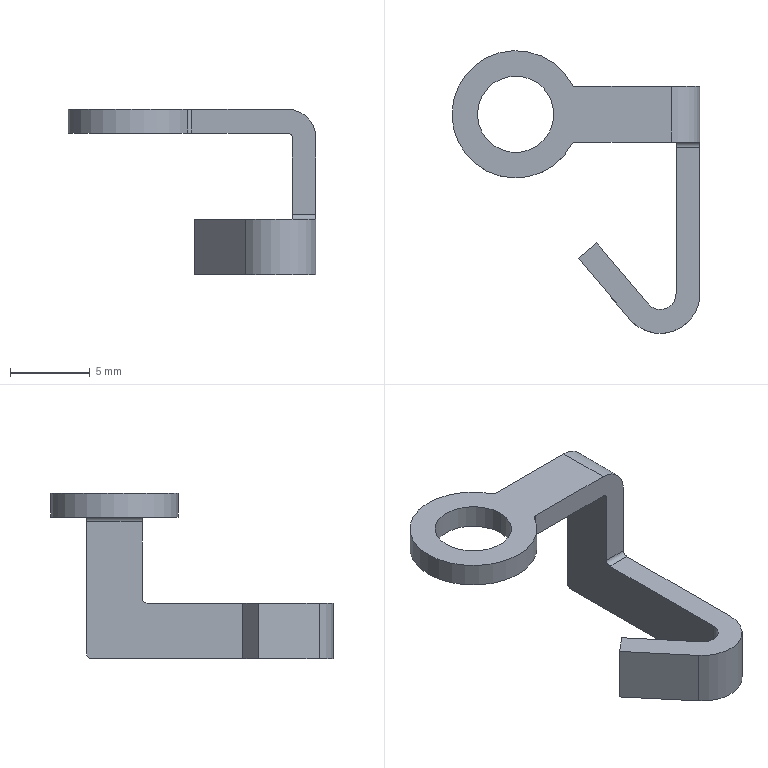Part | STEP file | TQ-DD-1105-THTerminalE1010_デフォルト | 1 solid | 22 faces | box 15.586 x 17.763 x 10.4 mm | volume 231.793 mm3 | cylinder 11 | plane 11 | commonest cylinder face diameters 0.6 x5 4.8 x2 2 x1 3.6 x1 5 x1 8 x1
STEP:
#1=CARTESIAN_POINT('',(2.4,0.,0.));
#2=VERTEX_POINT('',#1);
#3=CARTESIAN_POINT('',(-2.4,0.,0.));
#4=VERTEX_POINT('',#3);
#5=CARTESIAN_POINT('',(0.,0.,0.));
#6=DIRECTION('',(0.,0.,-1.));
#7=DIRECTION('',(1.,0.,0.));
#8=AXIS2_PLACEMENT_3D('',#5,#6,#7);
#9=CIRCLE('',#8,2.4);
#10=EDGE_CURVE('',#2,#4,#9,.T.);
#11=ORIENTED_EDGE('',*,*,#10,.T.);
#12=CARTESIAN_POINT('',(-2.4,0.,1.5));
#13=VERTEX_POINT('',#12);
#14=CARTESIAN_POINT('',(-2.4,0.,0.75));
#15=DIRECTION('',(0.,0.,1.));
#16=VECTOR('',#15,1000.);
#17=LINE('',#14,#16);
#18=EDGE_CURVE('',#4,#13,#17,.T.);
#19=ORIENTED_EDGE('',*,*,#18,.T.);
#20=CARTESIAN_POINT('',(2.4,0.,1.5));
#21=VERTEX_POINT('',#20);
#22=CARTESIAN_POINT('',(0.,0.,1.5));
#23=DIRECTION('',(0.,0.,-1.));
#24=DIRECTION('',(1.,0.,0.));
#25=AXIS2_PLACEMENT_3D('',#22,#23,#24);
#26=CIRCLE('',#25,2.4);
#27=EDGE_CURVE('',#21,#13,#26,.T.);
#28=ORIENTED_EDGE('',*,*,#27,.F.);
#29=CARTESIAN_POINT('',(2.4,0.,0.75));
#30=DIRECTION('',(0.,0.,1.));
#31=VECTOR('',#30,1000.);
#32=LINE('',#29,#31);
#33=EDGE_CURVE('',#2,#21,#32,.T.);
#34=ORIENTED_EDGE('',*,*,#33,.F.);
#35=EDGE_LOOP('',(#11,#19,#28,#34));
#36=FACE_OUTER_BOUND('',#35,.T.);
#37=CARTESIAN_POINT('',(0.,0.,0.75));
#38=DIRECTION('',(0.,0.,1.));
#39=DIRECTION('',(1.,0.,0.));
#40=AXIS2_PLACEMENT_3D('',#37,#38,#39);
#41=CYLINDRICAL_SURFACE('',#40,2.4);
#42=ADVANCED_FACE('',(#36),#41,.F.);
#43=CARTESIAN_POINT('',(10.086,-11.263,-8.9));
#44=VERTEX_POINT('',#43);
#45=CARTESIAN_POINT('',(10.086,1.45,-8.9));
#46=VERTEX_POINT('',#45);
#47=CARTESIAN_POINT('',(10.086,1.75,-8.9));
#48=DIRECTION('',(0.,1.,0.));
#49=VECTOR('',#48,1000.);
#50=LINE('',#47,#49);
#51=EDGE_CURVE('',#44,#46,#50,.T.);
#52=ORIENTED_EDGE('',*,*,#51,.F.);
#53=CARTESIAN_POINT('',(10.086,-11.263,-5.4));
#54=VERTEX_POINT('',#53);
#55=CARTESIAN_POINT('',(10.086,-11.263,-8.9));
#56=DIRECTION('',(0.,0.,-1.));
#57=VECTOR('',#56,1000.);
#58=LINE('',#55,#57);
#59=EDGE_CURVE('',#54,#44,#58,.T.);
#60=ORIENTED_EDGE('',*,*,#59,.F.);
#61=CARTESIAN_POINT('',(10.086,-2.05,-5.4));
#62=VERTEX_POINT('',#61);
#63=CARTESIAN_POINT('',(10.086,1.75,-5.4));
#64=DIRECTION('',(0.,-1.,0.));
#65=VECTOR('',#64,1000.);
#66=LINE('',#63,#65);
#67=EDGE_CURVE('',#62,#54,#66,.T.);
#68=ORIENTED_EDGE('',*,*,#67,.F.);
#69=CARTESIAN_POINT('',(10.086,-1.75,-5.1));
#70=VERTEX_POINT('',#69);
#71=CARTESIAN_POINT('',(10.086,-2.05,-5.1));
#72=DIRECTION('',(1.,0.,0.));
#73=DIRECTION('',(0.,0.,1.));
#74=AXIS2_PLACEMENT_3D('',#71,#72,#73);
#75=CIRCLE('',#74,0.3);
#76=EDGE_CURVE('',#62,#70,#75,.T.);
#77=ORIENTED_EDGE('',*,*,#76,.T.);
#78=CARTESIAN_POINT('',(10.086,-1.75,-0.3));
#79=VERTEX_POINT('',#78);
#80=CARTESIAN_POINT('',(10.086,-1.75,-8.9));
#81=DIRECTION('',(0.,0.,-1.));
#82=VECTOR('',#81,1000.);
#83=LINE('',#80,#82);
#84=EDGE_CURVE('',#79,#70,#83,.T.);
#85=ORIENTED_EDGE('',*,*,#84,.F.);
#86=CARTESIAN_POINT('',(10.086,1.75,-0.3));
#87=VERTEX_POINT('',#86);
#88=CARTESIAN_POINT('',(10.086,1.75,-0.3));
#89=DIRECTION('',(0.,-1.,0.));
#90=VECTOR('',#89,1000.);
#91=LINE('',#88,#90);
#92=EDGE_CURVE('',#87,#79,#91,.T.);
#93=ORIENTED_EDGE('',*,*,#92,.F.);
#94=CARTESIAN_POINT('',(10.086,1.75,-8.6));
#95=VERTEX_POINT('',#94);
#96=CARTESIAN_POINT('',(10.086,1.75,-8.9));
#97=DIRECTION('',(0.,0.,1.));
#98=VECTOR('',#97,1000.);
#99=LINE('',#96,#98);
#100=EDGE_CURVE('',#95,#87,#99,.T.);
#101=ORIENTED_EDGE('',*,*,#100,.F.);
#102=CARTESIAN_POINT('',(10.086,1.45,-8.6));
#103=DIRECTION('',(1.,0.,0.));
#104=DIRECTION('',(0.,0.,-1.));
#105=AXIS2_PLACEMENT_3D('',#102,#103,#104);
#106=CIRCLE('',#105,0.3);
#107=EDGE_CURVE('',#46,#95,#106,.T.);
#108=ORIENTED_EDGE('',*,*,#107,.F.);
#109=EDGE_LOOP('',(#52,#60,#68,#77,#85,#93,#101,#108));
#110=FACE_OUTER_BOUND('',#109,.T.);
#111=CARTESIAN_POINT('',(10.086,1.75,-8.9));
#112=DIRECTION('',(1.,0.,0.));
#113=DIRECTION('',(0.,0.,-1.));
#114=AXIS2_PLACEMENT_3D('',#111,#112,#113);
#115=PLANE('',#114);
#116=ADVANCED_FACE('',(#110),#115,.F.);
#117=ORIENTED_EDGE('',*,*,#51,.T.);
#118=CARTESIAN_POINT('',(11.586,1.45,-8.9));
#119=VERTEX_POINT('',#118);
#120=CARTESIAN_POINT('',(10.086,1.45,-8.9));
#121=DIRECTION('',(1.,0.,0.));
#122=VECTOR('',#121,1000.);
#123=LINE('',#120,#122);
#124=EDGE_CURVE('',#46,#119,#123,.T.);
#125=ORIENTED_EDGE('',*,*,#124,.T.);
#126=CARTESIAN_POINT('',(11.586,-11.263,-8.9));
#127=VERTEX_POINT('',#126);
#128=CARTESIAN_POINT('',(11.586,1.75,-8.9));
#129=DIRECTION('',(0.,-1.,0.));
#130=VECTOR('',#129,1000.);
#131=LINE('',#128,#130);
#132=EDGE_CURVE('',#119,#127,#131,.T.);
#133=ORIENTED_EDGE('',*,*,#132,.T.);
#134=CARTESIAN_POINT('',(7.171,-12.87,-8.9));
#135=VERTEX_POINT('',#134);
#136=CARTESIAN_POINT('',(9.086,-11.263,-8.9));
#137=DIRECTION('',(0.,0.,-1.));
#138=DIRECTION('',(1.,0.,0.));
#139=AXIS2_PLACEMENT_3D('',#136,#137,#138);
#140=CIRCLE('',#139,2.5);
#141=EDGE_CURVE('',#127,#135,#140,.T.);
#142=ORIENTED_EDGE('',*,*,#141,.T.);
#143=CARTESIAN_POINT('',(3.957,-9.04,-8.9));
#144=VERTEX_POINT('',#143);
#145=CARTESIAN_POINT('',(7.171,-12.87,-8.9));
#146=DIRECTION('',(-0.6428,0.766,0.));
#147=VECTOR('',#146,1000.);
#148=LINE('',#145,#147);
#149=EDGE_CURVE('',#135,#144,#148,.T.);
#150=ORIENTED_EDGE('',*,*,#149,.T.);
#151=CARTESIAN_POINT('',(5.106,-8.076,-8.9));
#152=VERTEX_POINT('',#151);
#153=CARTESIAN_POINT('',(3.957,-9.04,-8.9));
#154=DIRECTION('',(0.766,0.6428,0.));
#155=VECTOR('',#154,1000.);
#156=LINE('',#153,#155);
#157=EDGE_CURVE('',#144,#152,#156,.T.);
#158=ORIENTED_EDGE('',*,*,#157,.T.);
#159=CARTESIAN_POINT('',(8.32,-11.906,-8.9));
#160=VERTEX_POINT('',#159);
#161=CARTESIAN_POINT('',(5.106,-8.076,-8.9));
#162=DIRECTION('',(0.6428,-0.766,0.));
#163=VECTOR('',#162,1000.);
#164=LINE('',#161,#163);
#165=EDGE_CURVE('',#152,#160,#164,.T.);
#166=ORIENTED_EDGE('',*,*,#165,.T.);
#167=CARTESIAN_POINT('',(9.086,-11.263,-8.9));
#168=DIRECTION('',(0.,0.,1.));
#169=DIRECTION('',(1.,0.,0.));
#170=AXIS2_PLACEMENT_3D('',#167,#168,#169);
#171=CIRCLE('',#170,1.);
#172=EDGE_CURVE('',#160,#44,#171,.T.);
#173=ORIENTED_EDGE('',*,*,#172,.T.);
#174=EDGE_LOOP('',(#117,#125,#133,#142,#150,#158,#166,#173));
#175=FACE_OUTER_BOUND('',#174,.T.);
#176=CARTESIAN_POINT('',(10.086,1.75,-8.9));
#177=DIRECTION('',(0.,0.,-1.));
#178=DIRECTION('',(-1.,0.,0.));
#179=AXIS2_PLACEMENT_3D('',#176,#177,#178);
#180=PLANE('',#179);
#181=ADVANCED_FACE('',(#175),#180,.T.);
#182=ORIENTED_EDGE('',*,*,#172,.F.);
#183=CARTESIAN_POINT('',(8.32,-11.906,-5.4));
#184=VERTEX_POINT('',#183);
#185=CARTESIAN_POINT('',(8.32,-11.906,-7.15));
#186=DIRECTION('',(0.,0.,-1.));
#187=VECTOR('',#186,1000.);
#188=LINE('',#185,#187);
#189=EDGE_CURVE('',#184,#160,#188,.T.);
#190=ORIENTED_EDGE('',*,*,#189,.F.);
#191=CARTESIAN_POINT('',(9.086,-11.263,-5.4));
#192=DIRECTION('',(0.,0.,-1.));
#193=DIRECTION('',(1.,0.,0.));
#194=AXIS2_PLACEMENT_3D('',#191,#192,#193);
#195=CIRCLE('',#194,1.);
#196=EDGE_CURVE('',#54,#184,#195,.T.);
#197=ORIENTED_EDGE('',*,*,#196,.F.);
#198=ORIENTED_EDGE('',*,*,#59,.T.);
#199=EDGE_LOOP('',(#182,#190,#197,#198));
#200=FACE_OUTER_BOUND('',#199,.T.);
#201=CARTESIAN_POINT('',(9.086,-11.263,-7.15));
#202=DIRECTION('',(0.,0.,1.));
#203=DIRECTION('',(1.,0.,0.));
#204=AXIS2_PLACEMENT_3D('',#201,#202,#203);
#205=CYLINDRICAL_SURFACE('',#204,1.);
#206=ADVANCED_FACE('',(#200),#205,.F.);
#207=CARTESIAN_POINT('',(11.586,-11.263,-5.4));
#208=VERTEX_POINT('',#207);
#209=CARTESIAN_POINT('',(11.586,-2.05,-5.4));
#210=VERTEX_POINT('',#209);
#211=CARTESIAN_POINT('',(11.586,0.,-5.4));
#212=DIRECTION('',(0.,1.,0.));
#213=VECTOR('',#212,1000.);
#214=LINE('',#211,#213);
#215=EDGE_CURVE('',#208,#210,#214,.T.);
#216=ORIENTED_EDGE('',*,*,#215,.T.);
#217=CARTESIAN_POINT('',(0.,-2.05,-5.4));
#218=DIRECTION('',(-1.,0.,0.));
#219=VECTOR('',#218,1000.);
#220=LINE('',#217,#219);
#221=EDGE_CURVE('',#210,#62,#220,.T.);
#222=ORIENTED_EDGE('',*,*,#221,.T.);
#223=ORIENTED_EDGE('',*,*,#67,.T.);
#224=ORIENTED_EDGE('',*,*,#196,.T.);
#225=CARTESIAN_POINT('',(5.106,-8.076,-5.4));
#226=VERTEX_POINT('',#225);
#227=CARTESIAN_POINT('',(8.32,-11.906,-5.4));
#228=DIRECTION('',(-0.6428,0.766,0.));
#229=VECTOR('',#228,1000.);
#230=LINE('',#227,#229);
#231=EDGE_CURVE('',#184,#226,#230,.T.);
#232=ORIENTED_EDGE('',*,*,#231,.T.);
#233=CARTESIAN_POINT('',(3.957,-9.04,-5.4));
#234=VERTEX_POINT('',#233);
#235=CARTESIAN_POINT('',(3.957,-9.04,-5.4));
#236=DIRECTION('',(-0.766,-0.6428,0.));
#237=VECTOR('',#236,1000.);
#238=LINE('',#235,#237);
#239=EDGE_CURVE('',#226,#234,#238,.T.);
#240=ORIENTED_EDGE('',*,*,#239,.T.);
#241=CARTESIAN_POINT('',(7.171,-12.87,-5.4));
#242=VERTEX_POINT('',#241);
#243=CARTESIAN_POINT('',(3.957,-9.04,-5.4));
#244=DIRECTION('',(0.6428,-0.766,0.));
#245=VECTOR('',#244,1000.);
#246=LINE('',#243,#245);
#247=EDGE_CURVE('',#234,#242,#246,.T.);
#248=ORIENTED_EDGE('',*,*,#247,.T.);
#249=CARTESIAN_POINT('',(9.086,-11.263,-5.4));
#250=DIRECTION('',(0.,0.,1.));
#251=DIRECTION('',(1.,0.,0.));
#252=AXIS2_PLACEMENT_3D('',#249,#250,#251);
#253=CIRCLE('',#252,2.5);
#254=EDGE_CURVE('',#242,#208,#253,.T.);
#255=ORIENTED_EDGE('',*,*,#254,.T.);
#256=EDGE_LOOP('',(#216,#222,#223,#224,#232,#240,#248,#255));
#257=FACE_OUTER_BOUND('',#256,.T.);
#258=CARTESIAN_POINT('',(0.,0.,-5.4));
#259=DIRECTION('',(0.,0.,1.));
#260=DIRECTION('',(1.,0.,0.));
#261=AXIS2_PLACEMENT_3D('',#258,#259,#260);
#262=PLANE('',#261);
#263=ADVANCED_FACE('',(#257),#262,.T.);
#264=CARTESIAN_POINT('',(11.586,-1.75,-0.3));
#265=VERTEX_POINT('',#264);
#266=CARTESIAN_POINT('',(11.586,-1.75,-5.1));
#267=VERTEX_POINT('',#266);
#268=CARTESIAN_POINT('',(11.586,-1.75,0.));
#269=DIRECTION('',(0.,0.,-1.));
#270=VECTOR('',#269,1000.);
#271=LINE('',#268,#270);
#272=EDGE_CURVE('',#265,#267,#271,.T.);
#273=ORIENTED_EDGE('',*,*,#272,.F.);
#274=CARTESIAN_POINT('',(9.786,-1.75,1.5));
#275=VERTEX_POINT('',#274);
#276=CARTESIAN_POINT('',(9.786,-1.75,-0.3));
#277=DIRECTION('',(0.,1.,0.));
#278=DIRECTION('',(0.,0.,-1.));
#279=AXIS2_PLACEMENT_3D('',#276,#277,#278);
#280=CIRCLE('',#279,1.8);
#281=EDGE_CURVE('',#275,#265,#280,.T.);
#282=ORIENTED_EDGE('',*,*,#281,.F.);
#283=CARTESIAN_POINT('',(3.78,-1.75,1.5));
#284=VERTEX_POINT('',#283);
#285=CARTESIAN_POINT('',(11.586,-1.75,1.5));
#286=DIRECTION('',(1.,0.,0.));
#287=VECTOR('',#286,1000.);
#288=LINE('',#285,#287);
#289=EDGE_CURVE('',#284,#275,#288,.T.);
#290=ORIENTED_EDGE('',*,*,#289,.F.);
#291=CARTESIAN_POINT('',(3.78,-1.75,0.));
#292=VERTEX_POINT('',#291);
#293=CARTESIAN_POINT('',(3.78,-1.75,0.));
#294=DIRECTION('',(0.,0.,1.));
#295=VECTOR('',#294,1000.);
#296=LINE('',#293,#295);
#297=EDGE_CURVE('',#292,#284,#296,.T.);
#298=ORIENTED_EDGE('',*,*,#297,.F.);
#299=CARTESIAN_POINT('',(9.786,-1.75,0.));
#300=VERTEX_POINT('',#299);
#301=CARTESIAN_POINT('',(11.586,-1.75,0.));
#302=DIRECTION('',(-1.,0.,0.));
#303=VECTOR('',#302,1000.);
#304=LINE('',#301,#303);
#305=EDGE_CURVE('',#300,#292,#304,.T.);
#306=ORIENTED_EDGE('',*,*,#305,.F.);
#307=CARTESIAN_POINT('',(9.786,-1.75,-0.3));
#308=DIRECTION('',(0.,-1.,0.));
#309=DIRECTION('',(0.,0.,1.));
#310=AXIS2_PLACEMENT_3D('',#307,#308,#309);
#311=CIRCLE('',#310,0.3);
#312=EDGE_CURVE('',#79,#300,#311,.T.);
#313=ORIENTED_EDGE('',*,*,#312,.F.);
#314=ORIENTED_EDGE('',*,*,#84,.T.);
#315=CARTESIAN_POINT('',(11.586,-1.75,-5.1));
#316=DIRECTION('',(-1.,0.,0.));
#317=VECTOR('',#316,1000.);
#318=LINE('',#315,#317);
#319=EDGE_CURVE('',#267,#70,#318,.T.);
#320=ORIENTED_EDGE('',*,*,#319,.F.);
#321=EDGE_LOOP('',(#273,#282,#290,#298,#306,#313,#314,#320));
#322=FACE_OUTER_BOUND('',#321,.T.);
#323=CARTESIAN_POINT('',(11.586,-1.75,0.));
#324=DIRECTION('',(0.,1.,0.));
#325=DIRECTION('',(0.,0.,1.));
#326=AXIS2_PLACEMENT_3D('',#323,#324,#325);
#327=PLANE('',#326);
#328=ADVANCED_FACE('',(#322),#327,.F.);
#329=CARTESIAN_POINT('',(9.786,1.75,0.));
#330=VERTEX_POINT('',#329);
#331=CARTESIAN_POINT('',(9.786,1.75,-0.3));
#332=DIRECTION('',(0.,-1.,0.));
#333=DIRECTION('',(0.,0.,1.));
#334=AXIS2_PLACEMENT_3D('',#331,#332,#333);
#335=CIRCLE('',#334,0.3);
#336=EDGE_CURVE('',#87,#330,#335,.T.);
#337=ORIENTED_EDGE('',*,*,#336,.F.);
#338=ORIENTED_EDGE('',*,*,#92,.T.);
#339=ORIENTED_EDGE('',*,*,#312,.T.);
#340=CARTESIAN_POINT('',(9.786,0.,0.));
#341=DIRECTION('',(0.,-1.,0.));
#342=VECTOR('',#341,1000.);
#343=LINE('',#340,#342);
#344=EDGE_CURVE('',#330,#300,#343,.T.);
#345=ORIENTED_EDGE('',*,*,#344,.F.);
#346=EDGE_LOOP('',(#337,#338,#339,#345));
#347=FACE_OUTER_BOUND('',#346,.T.);
#348=CARTESIAN_POINT('',(9.786,0.,-0.3));
#349=DIRECTION('',(0.,1.,0.));
#350=DIRECTION('',(0.,0.,1.));
#351=AXIS2_PLACEMENT_3D('',#348,#349,#350);
#352=CYLINDRICAL_SURFACE('',#351,0.3);
#353=ADVANCED_FACE('',(#347),#352,.F.);
#354=ORIENTED_EDGE('',*,*,#100,.T.);
#355=ORIENTED_EDGE('',*,*,#336,.T.);
#356=CARTESIAN_POINT('',(3.78,1.75,0.));
#357=VERTEX_POINT('',#356);
#358=CARTESIAN_POINT('',(3.597,1.75,0.));
#359=DIRECTION('',(1.,0.,0.));
#360=VECTOR('',#359,1000.);
#361=LINE('',#358,#360);
#362=EDGE_CURVE('',#357,#330,#361,.T.);
#363=ORIENTED_EDGE('',*,*,#362,.F.);
#364=CARTESIAN_POINT('',(3.78,1.75,1.5));
#365=VERTEX_POINT('',#364);
#366=CARTESIAN_POINT('',(3.78,1.75,0.));
#367=DIRECTION('',(0.,0.,-1.));
#368=VECTOR('',#367,1000.);
#369=LINE('',#366,#368);
#370=EDGE_CURVE('',#365,#357,#369,.T.);
#371=ORIENTED_EDGE('',*,*,#370,.F.);
#372=CARTESIAN_POINT('',(9.786,1.75,1.5));
#373=VERTEX_POINT('',#372);
#374=CARTESIAN_POINT('',(3.597,1.75,1.5));
#375=DIRECTION('',(-1.,0.,0.));
#376=VECTOR('',#375,1000.);
#377=LINE('',#374,#376);
#378=EDGE_CURVE('',#373,#365,#377,.T.);
#379=ORIENTED_EDGE('',*,*,#378,.F.);
#380=CARTESIAN_POINT('',(11.586,1.75,-0.3));
#381=VERTEX_POINT('',#380);
#382=CARTESIAN_POINT('',(9.786,1.75,-0.3));
#383=DIRECTION('',(0.,-1.,0.));
#384=DIRECTION('',(0.,0.,-1.));
#385=AXIS2_PLACEMENT_3D('',#382,#383,#384);
#386=CIRCLE('',#385,1.8);
#387=EDGE_CURVE('',#381,#373,#386,.T.);
#388=ORIENTED_EDGE('',*,*,#387,.F.);
#389=CARTESIAN_POINT('',(11.586,1.75,-8.6));
#390=VERTEX_POINT('',#389);
#391=CARTESIAN_POINT('',(11.586,1.75,0.));
#392=DIRECTION('',(0.,0.,1.));
#393=VECTOR('',#392,1000.);
#394=LINE('',#391,#393);
#395=EDGE_CURVE('',#390,#381,#394,.T.);
#396=ORIENTED_EDGE('',*,*,#395,.F.);
#397=CARTESIAN_POINT('',(3.597,1.75,-8.6));
#398=DIRECTION('',(1.,0.,0.));
#399=VECTOR('',#398,1000.);
#400=LINE('',#397,#399);
#401=EDGE_CURVE('',#95,#390,#400,.T.);
#402=ORIENTED_EDGE('',*,*,#401,.F.);
#403=EDGE_LOOP('',(#354,#355,#363,#371,#379,#388,#396,#402));
#404=FACE_OUTER_BOUND('',#403,.T.);
#405=CARTESIAN_POINT('',(3.597,1.75,0.));
#406=DIRECTION('',(0.,-1.,0.));
#407=DIRECTION('',(0.,0.,-1.));
#408=AXIS2_PLACEMENT_3D('',#405,#406,#407);
#409=PLANE('',#408);
#410=ADVANCED_FACE('',(#404),#409,.F.);
#411=CARTESIAN_POINT('',(11.586,1.45,-8.6));
#412=DIRECTION('',(-1.,0.,0.));
#413=DIRECTION('',(0.,0.,-1.));
#414=AXIS2_PLACEMENT_3D('',#411,#412,#413);
#415=CIRCLE('',#414,0.3);
#416=EDGE_CURVE('',#390,#119,#415,.T.);
#417=ORIENTED_EDGE('',*,*,#416,.T.);
#418=ORIENTED_EDGE('',*,*,#124,.F.);
#419=ORIENTED_EDGE('',*,*,#107,.T.);
#420=ORIENTED_EDGE('',*,*,#401,.T.);
#421=EDGE_LOOP('',(#417,#418,#419,#420));
#422=FACE_OUTER_BOUND('',#421,.T.);
#423=CARTESIAN_POINT('',(7.683,1.45,-8.6));
#424=DIRECTION('',(1.,0.,0.));
#425=DIRECTION('',(0.,0.,-1.));
#426=AXIS2_PLACEMENT_3D('',#423,#424,#425);
#427=CYLINDRICAL_SURFACE('',#426,0.3);
#428=ADVANCED_FACE('',(#422),#427,.T.);
#429=CARTESIAN_POINT('',(5.106,-8.076,-8.9));
#430=DIRECTION('',(0.,0.,1.));
#431=VECTOR('',#430,1000.);
#432=LINE('',#429,#431);
#433=EDGE_CURVE('',#152,#226,#432,.T.);
#434=ORIENTED_EDGE('',*,*,#433,.T.);
#435=ORIENTED_EDGE('',*,*,#231,.F.);
#436=ORIENTED_EDGE('',*,*,#189,.T.);
#437=ORIENTED_EDGE('',*,*,#165,.F.);
#438=EDGE_LOOP('',(#434,#435,#436,#437));
#439=FACE_OUTER_BOUND('',#438,.T.);
#440=CARTESIAN_POINT('',(8.32,-11.906,-8.9));
#441=DIRECTION('',(0.766,0.6428,0.));
#442=DIRECTION('',(-0.6428,0.766,0.));
#443=AXIS2_PLACEMENT_3D('',#440,#441,#442);
#444=PLANE('',#443);
#445=ADVANCED_FACE('',(#439),#444,.T.);
#446=CARTESIAN_POINT('',(7.171,-12.87,-8.9));
#447=DIRECTION('',(0.,0.,1.));
#448=VECTOR('',#447,1000.);
#449=LINE('',#446,#448);
#450=EDGE_CURVE('',#135,#242,#449,.T.);
#451=ORIENTED_EDGE('',*,*,#450,.T.);
#452=ORIENTED_EDGE('',*,*,#247,.F.);
#453=CARTESIAN_POINT('',(3.957,-9.04,-8.9));
#454=DIRECTION('',(0.,0.,-1.));
#455=VECTOR('',#454,1000.);
#456=LINE('',#453,#455);
#457=EDGE_CURVE('',#234,#144,#456,.T.);
#458=ORIENTED_EDGE('',*,*,#457,.T.);
#459=ORIENTED_EDGE('',*,*,#149,.F.);
#460=EDGE_LOOP('',(#451,#452,#458,#459));
#461=FACE_OUTER_BOUND('',#460,.T.);
#462=CARTESIAN_POINT('',(3.957,-9.04,-8.9));
#463=DIRECTION('',(-0.766,-0.6428,0.));
#464=DIRECTION('',(0.6428,-0.766,0.));
#465=AXIS2_PLACEMENT_3D('',#462,#463,#464);
#466=PLANE('',#465);
#467=ADVANCED_FACE('',(#461),#466,.T.);
#468=CARTESIAN_POINT('',(11.586,-11.263,-7.15));
#469=DIRECTION('',(0.,0.,1.));
#470=VECTOR('',#469,1000.);
#471=LINE('',#468,#470);
#472=EDGE_CURVE('',#127,#208,#471,.T.);
#473=ORIENTED_EDGE('',*,*,#472,.T.);
#474=ORIENTED_EDGE('',*,*,#254,.F.);
#475=ORIENTED_EDGE('',*,*,#450,.F.);
#476=ORIENTED_EDGE('',*,*,#141,.F.);
#477=EDGE_LOOP('',(#473,#474,#475,#476));
#478=FACE_OUTER_BOUND('',#477,.T.);
#479=CARTESIAN_POINT('',(9.086,-11.263,-7.15));
#480=DIRECTION('',(0.,0.,1.));
#481=DIRECTION('',(1.,0.,0.));
#482=AXIS2_PLACEMENT_3D('',#479,#480,#481);
#483=CYLINDRICAL_SURFACE('',#482,2.5);
#484=ADVANCED_FACE('',(#478),#483,.T.);
#485=ORIENTED_EDGE('',*,*,#395,.T.);
#486=CARTESIAN_POINT('',(11.586,1.75,-0.3));
#487=DIRECTION('',(0.,1.,0.));
#488=VECTOR('',#487,1000.);
#489=LINE('',#486,#488);
#490=EDGE_CURVE('',#265,#381,#489,.T.);
#491=ORIENTED_EDGE('',*,*,#490,.F.);
#492=ORIENTED_EDGE('',*,*,#272,.T.);
#493=CARTESIAN_POINT('',(11.586,-2.05,-5.1));
#494=DIRECTION('',(1.,0.,0.));
#495=DIRECTION('',(0.,0.,1.));
#496=AXIS2_PLACEMENT_3D('',#493,#494,#495);
#497=CIRCLE('',#496,0.3);
#498=EDGE_CURVE('',#210,#267,#497,.T.);
#499=ORIENTED_EDGE('',*,*,#498,.F.);
#500=ORIENTED_EDGE('',*,*,#215,.F.);
#501=ORIENTED_EDGE('',*,*,#472,.F.);
#502=ORIENTED_EDGE('',*,*,#132,.F.);
#503=ORIENTED_EDGE('',*,*,#416,.F.);
#504=EDGE_LOOP('',(#485,#491,#492,#499,#500,#501,#502,#503));
#505=FACE_OUTER_BOUND('',#504,.T.);
#506=CARTESIAN_POINT('',(11.586,1.75,0.));
#507=DIRECTION('',(-1.,0.,0.));
#508=DIRECTION('',(0.,0.,1.));
#509=AXIS2_PLACEMENT_3D('',#506,#507,#508);
#510=PLANE('',#509);
#511=ADVANCED_FACE('',(#505),#510,.F.);
#512=ORIENTED_EDGE('',*,*,#76,.F.);
#513=ORIENTED_EDGE('',*,*,#221,.F.);
#514=ORIENTED_EDGE('',*,*,#498,.T.);
#515=ORIENTED_EDGE('',*,*,#319,.T.);
#516=EDGE_LOOP('',(#512,#513,#514,#515));
#517=FACE_OUTER_BOUND('',#516,.T.);
#518=CARTESIAN_POINT('',(7.683,-2.05,-5.1));
#519=DIRECTION('',(-1.,0.,0.));
#520=DIRECTION('',(0.,0.,1.));
#521=AXIS2_PLACEMENT_3D('',#518,#519,#520);
#522=CYLINDRICAL_SURFACE('',#521,0.3);
#523=ADVANCED_FACE('',(#517),#522,.F.);
#524=ORIENTED_EDGE('',*,*,#387,.T.);
#525=CARTESIAN_POINT('',(9.786,0.,1.5));
#526=DIRECTION('',(0.,-1.,0.));
#527=VECTOR('',#526,1000.);
#528=LINE('',#525,#527);
#529=EDGE_CURVE('',#373,#275,#528,.T.);
#530=ORIENTED_EDGE('',*,*,#529,.T.);
#531=ORIENTED_EDGE('',*,*,#281,.T.);
#532=ORIENTED_EDGE('',*,*,#490,.T.);
#533=EDGE_LOOP('',(#524,#530,#531,#532));
#534=FACE_OUTER_BOUND('',#533,.T.);
#535=CARTESIAN_POINT('',(9.786,0.,-0.3));
#536=DIRECTION('',(0.,-1.,0.));
#537=DIRECTION('',(0.,0.,-1.));
#538=AXIS2_PLACEMENT_3D('',#535,#536,#537);
#539=CYLINDRICAL_SURFACE('',#538,1.8);
#540=ADVANCED_FACE('',(#534),#539,.T.);
#541=ORIENTED_EDGE('',*,*,#27,.T.);
#542=CARTESIAN_POINT('',(0.,0.,1.5));
#543=DIRECTION('',(0.,0.,-1.));
#544=DIRECTION('',(1.,0.,0.));
#545=AXIS2_PLACEMENT_3D('',#542,#543,#544);
#546=CIRCLE('',#545,2.4);
#547=EDGE_CURVE('',#13,#21,#546,.T.);
#548=ORIENTED_EDGE('',*,*,#547,.T.);
#549=EDGE_LOOP('',(#541,#548));
#550=FACE_BOUND('',#549,.T.);
#551=ORIENTED_EDGE('',*,*,#529,.F.);
#552=ORIENTED_EDGE('',*,*,#378,.T.);
#553=CARTESIAN_POINT('',(3.516,1.907,1.5));
#554=VERTEX_POINT('',#553);
#555=CARTESIAN_POINT('',(3.78,2.05,1.5));
#556=DIRECTION('',(0.,0.,-1.));
#557=DIRECTION('',(-1.,0.,0.));
#558=AXIS2_PLACEMENT_3D('',#555,#556,#557);
#559=CIRCLE('',#558,0.3);
#560=EDGE_CURVE('',#365,#554,#559,.T.);
#561=ORIENTED_EDGE('',*,*,#560,.T.);
#562=CARTESIAN_POINT('',(3.516,-1.907,1.5));
#563=VERTEX_POINT('',#562);
#564=CARTESIAN_POINT('',(0.,0.,1.5));
#565=DIRECTION('',(0.,0.,1.));
#566=DIRECTION('',(1.,0.,0.));
#567=AXIS2_PLACEMENT_3D('',#564,#565,#566);
#568=CIRCLE('',#567,4.);
#569=EDGE_CURVE('',#554,#563,#568,.T.);
#570=ORIENTED_EDGE('',*,*,#569,.T.);
#571=CARTESIAN_POINT('',(3.78,-2.05,1.5));
#572=DIRECTION('',(0.,0.,-1.));
#573=DIRECTION('',(-1.,0.,0.));
#574=AXIS2_PLACEMENT_3D('',#571,#572,#573);
#575=CIRCLE('',#574,0.3);
#576=EDGE_CURVE('',#563,#284,#575,.T.);
#577=ORIENTED_EDGE('',*,*,#576,.T.);
#578=ORIENTED_EDGE('',*,*,#289,.T.);
#579=EDGE_LOOP('',(#551,#552,#561,#570,#577,#578));
#580=FACE_OUTER_BOUND('',#579,.T.);
#581=CARTESIAN_POINT('',(0.,0.,1.5));
#582=DIRECTION('',(0.,0.,1.));
#583=DIRECTION('',(1.,0.,0.));
#584=AXIS2_PLACEMENT_3D('',#581,#582,#583);
#585=PLANE('',#584);
#586=ADVANCED_FACE('',(#550,#580),#585,.T.);
#587=ORIENTED_EDGE('',*,*,#576,.F.);
#588=CARTESIAN_POINT('',(3.516,-1.907,0.));
#589=VERTEX_POINT('',#588);
#590=CARTESIAN_POINT('',(3.516,-1.907,-3.7));
#591=DIRECTION('',(0.,0.,1.));
#592=VECTOR('',#591,1000.);
#593=LINE('',#590,#592);
#594=EDGE_CURVE('',#589,#563,#593,.T.);
#595=ORIENTED_EDGE('',*,*,#594,.F.);
#596=CARTESIAN_POINT('',(3.78,-2.05,0.));
#597=DIRECTION('',(0.,0.,1.));
#598=DIRECTION('',(-1.,0.,0.));
#599=AXIS2_PLACEMENT_3D('',#596,#597,#598);
#600=CIRCLE('',#599,0.3);
#601=EDGE_CURVE('',#292,#589,#600,.T.);
#602=ORIENTED_EDGE('',*,*,#601,.F.);
#603=ORIENTED_EDGE('',*,*,#297,.T.);
#604=EDGE_LOOP('',(#587,#595,#602,#603));
#605=FACE_OUTER_BOUND('',#604,.T.);
#606=CARTESIAN_POINT('',(3.78,-2.05,-3.7));
#607=DIRECTION('',(0.,0.,-1.));
#608=DIRECTION('',(-1.,0.,0.));
#609=AXIS2_PLACEMENT_3D('',#606,#607,#608);
#610=CYLINDRICAL_SURFACE('',#609,0.3);
#611=ADVANCED_FACE('',(#605),#610,.F.);
#612=ORIENTED_EDGE('',*,*,#10,.F.);
#613=CARTESIAN_POINT('',(0.,0.,0.));
#614=DIRECTION('',(0.,0.,-1.));
#615=DIRECTION('',(1.,0.,0.));
#616=AXIS2_PLACEMENT_3D('',#613,#614,#615);
#617=CIRCLE('',#616,2.4);
#618=EDGE_CURVE('',#4,#2,#617,.T.);
#619=ORIENTED_EDGE('',*,*,#618,.F.);
#620=EDGE_LOOP('',(#612,#619));
#621=FACE_BOUND('',#620,.T.);
#622=ORIENTED_EDGE('',*,*,#344,.T.);
#623=ORIENTED_EDGE('',*,*,#305,.T.);
#624=ORIENTED_EDGE('',*,*,#601,.T.);
#625=CARTESIAN_POINT('',(3.516,1.907,0.));
#626=VERTEX_POINT('',#625);
#627=CARTESIAN_POINT('',(0.,0.,0.));
#628=DIRECTION('',(0.,0.,1.));
#629=DIRECTION('',(1.,0.,0.));
#630=AXIS2_PLACEMENT_3D('',#627,#628,#629);
#631=CIRCLE('',#630,4.);
#632=EDGE_CURVE('',#626,#589,#631,.T.);
#633=ORIENTED_EDGE('',*,*,#632,.F.);
#634=CARTESIAN_POINT('',(3.78,2.05,0.));
#635=DIRECTION('',(0.,0.,-1.));
#636=DIRECTION('',(-1.,0.,0.));
#637=AXIS2_PLACEMENT_3D('',#634,#635,#636);
#638=CIRCLE('',#637,0.3);
#639=EDGE_CURVE('',#357,#626,#638,.T.);
#640=ORIENTED_EDGE('',*,*,#639,.F.);
#641=ORIENTED_EDGE('',*,*,#362,.T.);
#642=EDGE_LOOP('',(#622,#623,#624,#633,#640,#641));
#643=FACE_OUTER_BOUND('',#642,.T.);
#644=CARTESIAN_POINT('',(0.,0.,0.));
#645=DIRECTION('',(0.,0.,1.));
#646=DIRECTION('',(1.,0.,0.));
#647=AXIS2_PLACEMENT_3D('',#644,#645,#646);
#648=PLANE('',#647);
#649=ADVANCED_FACE('',(#621,#643),#648,.F.);
#650=ORIENTED_EDGE('',*,*,#560,.F.);
#651=ORIENTED_EDGE('',*,*,#370,.T.);
#652=ORIENTED_EDGE('',*,*,#639,.T.);
#653=CARTESIAN_POINT('',(3.516,1.907,-3.7));
#654=DIRECTION('',(0.,0.,-1.));
#655=VECTOR('',#654,1000.);
#656=LINE('',#653,#655);
#657=EDGE_CURVE('',#554,#626,#656,.T.);
#658=ORIENTED_EDGE('',*,*,#657,.F.);
#659=EDGE_LOOP('',(#650,#651,#652,#658));
#660=FACE_OUTER_BOUND('',#659,.T.);
#661=CARTESIAN_POINT('',(3.78,2.05,-3.7));
#662=DIRECTION('',(0.,0.,-1.));
#663=DIRECTION('',(-1.,0.,0.));
#664=AXIS2_PLACEMENT_3D('',#661,#662,#663);
#665=CYLINDRICAL_SURFACE('',#664,0.3);
#666=ADVANCED_FACE('',(#660),#665,.F.);
#667=ORIENTED_EDGE('',*,*,#157,.F.);
#668=ORIENTED_EDGE('',*,*,#457,.F.);
#669=ORIENTED_EDGE('',*,*,#239,.F.);
#670=ORIENTED_EDGE('',*,*,#433,.F.);
#671=EDGE_LOOP('',(#667,#668,#669,#670));
#672=FACE_OUTER_BOUND('',#671,.T.);
#673=CARTESIAN_POINT('',(3.957,-9.04,-8.9));
#674=DIRECTION('',(0.6428,-0.766,0.));
#675=DIRECTION('',(0.766,0.6428,0.));
#676=AXIS2_PLACEMENT_3D('',#673,#674,#675);
#677=PLANE('',#676);
#678=ADVANCED_FACE('',(#672),#677,.F.);
#679=ORIENTED_EDGE('',*,*,#18,.F.);
#680=ORIENTED_EDGE('',*,*,#618,.T.);
#681=ORIENTED_EDGE('',*,*,#33,.T.);
#682=ORIENTED_EDGE('',*,*,#547,.F.);
#683=EDGE_LOOP('',(#679,#680,#681,#682));
#684=FACE_OUTER_BOUND('',#683,.T.);
#685=CARTESIAN_POINT('',(0.,0.,0.75));
#686=DIRECTION('',(0.,0.,1.));
#687=DIRECTION('',(1.,0.,0.));
#688=AXIS2_PLACEMENT_3D('',#685,#686,#687);
#689=CYLINDRICAL_SURFACE('',#688,2.4);
#690=ADVANCED_FACE('',(#684),#689,.F.);
#691=ORIENTED_EDGE('',*,*,#569,.F.);
#692=ORIENTED_EDGE('',*,*,#657,.T.);
#693=ORIENTED_EDGE('',*,*,#632,.T.);
#694=ORIENTED_EDGE('',*,*,#594,.T.);
#695=EDGE_LOOP('',(#691,#692,#693,#694));
#696=FACE_OUTER_BOUND('',#695,.T.);
#697=CARTESIAN_POINT('',(0.,0.,0.75));
#698=DIRECTION('',(0.,0.,1.));
#699=DIRECTION('',(1.,0.,0.));
#700=AXIS2_PLACEMENT_3D('',#697,#698,#699);
#701=CYLINDRICAL_SURFACE('',#700,4.);
#702=ADVANCED_FACE('',(#696),#701,.T.);
#703=CLOSED_SHELL('',(#42,#116,#181,#206,#263,#328,#353,#410,#428,#445,#467,#484,#511,#523,#540,#586,#611,#649,#666,#678,#690,#702));
#704=MANIFOLD_SOLID_BREP('',#703);
#705=CARTESIAN_POINT('',(0.,0.,0.));
#706=DIRECTION('',(0.,0.,1.));
#707=DIRECTION('',(1.,0.,0.));
#708=AXIS2_PLACEMENT_3D('',#705,#706,#707);
#709=(LENGTH_UNIT()NAMED_UNIT(*)SI_UNIT(.MILLI.,.METRE.));
#710=UNCERTAINTY_MEASURE_WITH_UNIT(LENGTH_MEASURE(0.00001),#709,'','');
#711=(NAMED_UNIT(*)PLANE_ANGLE_UNIT()SI_UNIT($,.RADIAN.));
#712=(NAMED_UNIT(*)SI_UNIT($,.STERADIAN.)SOLID_ANGLE_UNIT());
#713=(GEOMETRIC_REPRESENTATION_CONTEXT(3)GLOBAL_UNCERTAINTY_ASSIGNED_CONTEXT((#710))GLOBAL_UNIT_ASSIGNED_CONTEXT((#709,#711,#712))REPRESENTATION_CONTEXT('',''));
#714=ADVANCED_BREP_SHAPE_REPRESENTATION('',(#704,#708),#713);